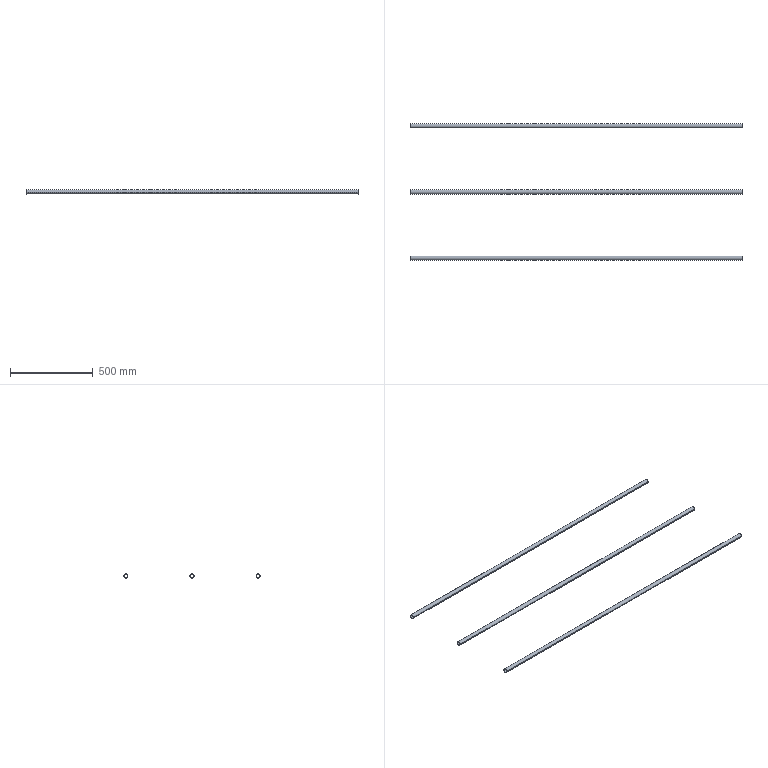Part | STEP file | E3-Transfer kettle guardrail 3 rail_Default<As Machined> | 3 solids | 18 faces | box 2008 x 825 x 25 mm | volume 667105 mm3 | cylinder 12 | plane 6 | commonest cylinder face diameters 22 x6 25 x6
STEP:
#1=CARTESIAN_POINT('',(0.,0.,0.));
#2=DIRECTION('',(0.,0.,1.));
#3=DIRECTION('',(1.,0.,0.));
#4=AXIS2_PLACEMENT_3D('',#1,#2,#3);
#5=CARTESIAN_POINT('',(1004.,787.5,0.));
#6=VERTEX_POINT('',#5);
#7=CARTESIAN_POINT('',(1004.,812.5,0.));
#8=VERTEX_POINT('',#7);
#9=CARTESIAN_POINT('',(1004.,800.,0.));
#10=DIRECTION('',(-1.,0.,0.));
#11=DIRECTION('',(0.,1.,0.));
#12=AXIS2_PLACEMENT_3D('',#9,#10,#11);
#13=CIRCLE('',#12,12.5);
#14=CARTESIAN_POINT('',(1004.,800.,0.));
#15=DIRECTION('',(-1.,0.,0.));
#16=DIRECTION('',(0.,-1.,0.));
#17=AXIS2_PLACEMENT_3D('',#14,#15,#16);
#18=CYLINDRICAL_SURFACE('',#17,12.5);
#19=CARTESIAN_POINT('',(-3.142,0.));
#20=DIRECTION('',(1.,0.));
#21=VECTOR('',#20,1.);
#22=LINE('',#19,#21);
#23=(GEOMETRIC_REPRESENTATION_CONTEXT(2)PARAMETRIC_REPRESENTATION_CONTEXT()REPRESENTATION_CONTEXT('',''));
#24=DEFINITIONAL_REPRESENTATION('',(#22),#23);
#25=PCURVE('',#18,#24);
#26=CARTESIAN_POINT('',(1004.,800.,0.));
#27=DIRECTION('',(1.,0.,0.));
#28=DIRECTION('',(0.,1.,0.));
#29=AXIS2_PLACEMENT_3D('',#26,#27,#28);
#30=PLANE('',#29);
#31=CARTESIAN_POINT('',(12.5,0.));
#32=CARTESIAN_POINT('',(12.5,-21.651));
#33=CARTESIAN_POINT('',(-6.25,-10.825));
#34=CARTESIAN_POINT('',(-25.,0.));
#35=CARTESIAN_POINT('',(-6.25,10.825));
#36=CARTESIAN_POINT('',(12.5,21.651));
#37=CARTESIAN_POINT('',(12.5,0.));
#38=(BOUNDED_CURVE()B_SPLINE_CURVE(2,(#31,#32,#33,#34,#35,#36,#37),.UNSPECIFIED.,.T.,.F.)B_SPLINE_CURVE_WITH_KNOTS((1,2,2,2,2,1),(-2.094,0.,2.094,4.189,6.283,8.378),.UNSPECIFIED.)CURVE()GEOMETRIC_REPRESENTATION_ITEM()RATIONAL_B_SPLINE_CURVE((1.,0.5,1.,0.5,1.,0.5,1.))REPRESENTATION_ITEM(''));
#39=(GEOMETRIC_REPRESENTATION_CONTEXT(2)PARAMETRIC_REPRESENTATION_CONTEXT()REPRESENTATION_CONTEXT('',''));
#40=DEFINITIONAL_REPRESENTATION('',(#38),#39);
#41=PCURVE('',#30,#40);
#42=SURFACE_CURVE('',#13,(#25,#41),.PCURVE_S1.);
#43=EDGE_CURVE('',#6,#8,#42,.T.);
#44=ORIENTED_EDGE('',*,*,#43,.T.);
#45=CARTESIAN_POINT('',(-1004.,812.5,0.));
#46=VERTEX_POINT('',#45);
#47=CARTESIAN_POINT('',(1004.,812.5,0.));
#48=DIRECTION('',(-1.,0.,0.));
#49=VECTOR('',#48,1.);
#50=LINE('',#47,#49);
#51=CARTESIAN_POINT('',(3.142,0.));
#52=DIRECTION('',(0.,1.));
#53=VECTOR('',#52,1.);
#54=LINE('',#51,#53);
#55=(GEOMETRIC_REPRESENTATION_CONTEXT(2)PARAMETRIC_REPRESENTATION_CONTEXT()REPRESENTATION_CONTEXT('',''));
#56=DEFINITIONAL_REPRESENTATION('',(#54),#55);
#57=PCURVE('',#18,#56);
#58=CARTESIAN_POINT('',(1004.,800.,0.));
#59=DIRECTION('',(-1.,0.,0.));
#60=DIRECTION('',(0.,-1.,0.));
#61=AXIS2_PLACEMENT_3D('',#58,#59,#60);
#62=CYLINDRICAL_SURFACE('',#61,12.5);
#63=CARTESIAN_POINT('',(3.142,0.));
#64=DIRECTION('',(0.,1.));
#65=VECTOR('',#64,1.);
#66=LINE('',#63,#65);
#67=(GEOMETRIC_REPRESENTATION_CONTEXT(2)PARAMETRIC_REPRESENTATION_CONTEXT()REPRESENTATION_CONTEXT('',''));
#68=DEFINITIONAL_REPRESENTATION('',(#66),#67);
#69=PCURVE('',#62,#68);
#70=SURFACE_CURVE('',#50,(#57,#69),.PCURVE_S1.);
#71=EDGE_CURVE('',#8,#46,#70,.T.);
#72=ORIENTED_EDGE('',*,*,#71,.T.);
#73=CARTESIAN_POINT('',(-1004.,787.5,0.));
#74=VERTEX_POINT('',#73);
#75=CARTESIAN_POINT('',(-1004.,800.,0.));
#76=DIRECTION('',(-1.,0.,0.));
#77=DIRECTION('',(0.,1.,0.));
#78=AXIS2_PLACEMENT_3D('',#75,#76,#77);
#79=CIRCLE('',#78,12.5);
#80=CARTESIAN_POINT('',(-3.142,2008.));
#81=DIRECTION('',(1.,0.));
#82=VECTOR('',#81,1.);
#83=LINE('',#80,#82);
#84=(GEOMETRIC_REPRESENTATION_CONTEXT(2)PARAMETRIC_REPRESENTATION_CONTEXT()REPRESENTATION_CONTEXT('',''));
#85=DEFINITIONAL_REPRESENTATION('',(#83),#84);
#86=PCURVE('',#18,#85);
#87=CARTESIAN_POINT('',(-1004.,800.,0.));
#88=DIRECTION('',(1.,0.,0.));
#89=DIRECTION('',(0.,1.,0.));
#90=AXIS2_PLACEMENT_3D('',#87,#88,#89);
#91=PLANE('',#90);
#92=CARTESIAN_POINT('',(12.5,0.));
#93=CARTESIAN_POINT('',(12.5,-21.651));
#94=CARTESIAN_POINT('',(-6.25,-10.825));
#95=CARTESIAN_POINT('',(-25.,0.));
#96=CARTESIAN_POINT('',(-6.25,10.825));
#97=CARTESIAN_POINT('',(12.5,21.651));
#98=CARTESIAN_POINT('',(12.5,0.));
#99=(BOUNDED_CURVE()B_SPLINE_CURVE(2,(#92,#93,#94,#95,#96,#97,#98),.UNSPECIFIED.,.T.,.F.)B_SPLINE_CURVE_WITH_KNOTS((1,2,2,2,2,1),(-2.094,0.,2.094,4.189,6.283,8.378),.UNSPECIFIED.)CURVE()GEOMETRIC_REPRESENTATION_ITEM()RATIONAL_B_SPLINE_CURVE((1.,0.5,1.,0.5,1.,0.5,1.))REPRESENTATION_ITEM(''));
#100=(GEOMETRIC_REPRESENTATION_CONTEXT(2)PARAMETRIC_REPRESENTATION_CONTEXT()REPRESENTATION_CONTEXT('',''));
#101=DEFINITIONAL_REPRESENTATION('',(#99),#100);
#102=PCURVE('',#91,#101);
#103=SURFACE_CURVE('',#79,(#86,#102),.PCURVE_S1.);
#104=EDGE_CURVE('',#74,#46,#103,.T.);
#105=ORIENTED_EDGE('',*,*,#104,.F.);
#106=CARTESIAN_POINT('',(1004.,787.5,0.));
#107=DIRECTION('',(-1.,0.,0.));
#108=VECTOR('',#107,1.);
#109=LINE('',#106,#108);
#110=CARTESIAN_POINT('',(0.,0.));
#111=DIRECTION('',(0.,1.));
#112=VECTOR('',#111,1.);
#113=LINE('',#110,#112);
#114=(GEOMETRIC_REPRESENTATION_CONTEXT(2)PARAMETRIC_REPRESENTATION_CONTEXT()REPRESENTATION_CONTEXT('',''));
#115=DEFINITIONAL_REPRESENTATION('',(#113),#114);
#116=PCURVE('',#18,#115);
#117=CARTESIAN_POINT('',(6.283,0.));
#118=DIRECTION('',(0.,1.));
#119=VECTOR('',#118,1.);
#120=LINE('',#117,#119);
#121=(GEOMETRIC_REPRESENTATION_CONTEXT(2)PARAMETRIC_REPRESENTATION_CONTEXT()REPRESENTATION_CONTEXT('',''));
#122=DEFINITIONAL_REPRESENTATION('',(#120),#121);
#123=PCURVE('',#62,#122);
#124=SURFACE_CURVE('',#109,(#116,#123),.PCURVE_S1.);
#125=EDGE_CURVE('',#6,#74,#124,.T.);
#126=ORIENTED_EDGE('',*,*,#125,.F.);
#127=EDGE_LOOP('',(#44,#72,#105,#126));
#128=FACE_BOUND('',#127,.T.);
#129=ADVANCED_FACE('',(#128),#18,.T.);
#130=CARTESIAN_POINT('',(1004.,789.,0.));
#131=VERTEX_POINT('',#130);
#132=CARTESIAN_POINT('',(-1004.,789.,0.));
#133=VERTEX_POINT('',#132);
#134=CARTESIAN_POINT('',(1004.,789.,0.));
#135=DIRECTION('',(-1.,0.,0.));
#136=VECTOR('',#135,1.);
#137=LINE('',#134,#136);
#138=CARTESIAN_POINT('',(1004.,800.,0.));
#139=DIRECTION('',(-1.,0.,0.));
#140=DIRECTION('',(0.,-1.,0.));
#141=AXIS2_PLACEMENT_3D('',#138,#139,#140);
#142=CYLINDRICAL_SURFACE('',#141,11.);
#143=CARTESIAN_POINT('',(6.283,0.));
#144=DIRECTION('',(0.,1.));
#145=VECTOR('',#144,1.);
#146=LINE('',#143,#145);
#147=(GEOMETRIC_REPRESENTATION_CONTEXT(2)PARAMETRIC_REPRESENTATION_CONTEXT()REPRESENTATION_CONTEXT('',''));
#148=DEFINITIONAL_REPRESENTATION('',(#146),#147);
#149=PCURVE('',#142,#148);
#150=CARTESIAN_POINT('',(1004.,800.,0.));
#151=DIRECTION('',(-1.,0.,0.));
#152=DIRECTION('',(0.,-1.,0.));
#153=AXIS2_PLACEMENT_3D('',#150,#151,#152);
#154=CYLINDRICAL_SURFACE('',#153,11.);
#155=CARTESIAN_POINT('',(0.,0.));
#156=DIRECTION('',(0.,1.));
#157=VECTOR('',#156,1.);
#158=LINE('',#155,#157);
#159=(GEOMETRIC_REPRESENTATION_CONTEXT(2)PARAMETRIC_REPRESENTATION_CONTEXT()REPRESENTATION_CONTEXT('',''));
#160=DEFINITIONAL_REPRESENTATION('',(#158),#159);
#161=PCURVE('',#154,#160);
#162=SURFACE_CURVE('',#137,(#149,#161),.PCURVE_S1.);
#163=EDGE_CURVE('',#131,#133,#162,.T.);
#164=ORIENTED_EDGE('',*,*,#163,.T.);
#165=CARTESIAN_POINT('',(-1004.,811.,0.));
#166=VERTEX_POINT('',#165);
#167=CARTESIAN_POINT('',(-1004.,800.,0.));
#168=DIRECTION('',(-1.,0.,0.));
#169=DIRECTION('',(0.,1.,0.));
#170=AXIS2_PLACEMENT_3D('',#167,#168,#169);
#171=CIRCLE('',#170,11.);
#172=CARTESIAN_POINT('',(3.142,2008.));
#173=DIRECTION('',(1.,0.));
#174=VECTOR('',#173,1.);
#175=LINE('',#172,#174);
#176=(GEOMETRIC_REPRESENTATION_CONTEXT(2)PARAMETRIC_REPRESENTATION_CONTEXT()REPRESENTATION_CONTEXT('',''));
#177=DEFINITIONAL_REPRESENTATION('',(#175),#176);
#178=PCURVE('',#142,#177);
#179=CARTESIAN_POINT('',(11.,0.));
#180=CARTESIAN_POINT('',(11.,-19.053));
#181=CARTESIAN_POINT('',(-5.5,-9.526));
#182=CARTESIAN_POINT('',(-22.,0.));
#183=CARTESIAN_POINT('',(-5.5,9.526));
#184=CARTESIAN_POINT('',(11.,19.053));
#185=CARTESIAN_POINT('',(11.,0.));
#186=(BOUNDED_CURVE()B_SPLINE_CURVE(2,(#179,#180,#181,#182,#183,#184,#185),.UNSPECIFIED.,.T.,.F.)B_SPLINE_CURVE_WITH_KNOTS((1,2,2,2,2,1),(-2.094,0.,2.094,4.189,6.283,8.378),.UNSPECIFIED.)CURVE()GEOMETRIC_REPRESENTATION_ITEM()RATIONAL_B_SPLINE_CURVE((1.,0.5,1.,0.5,1.,0.5,1.))REPRESENTATION_ITEM(''));
#187=(GEOMETRIC_REPRESENTATION_CONTEXT(2)PARAMETRIC_REPRESENTATION_CONTEXT()REPRESENTATION_CONTEXT('',''));
#188=DEFINITIONAL_REPRESENTATION('',(#186),#187);
#189=PCURVE('',#91,#188);
#190=SURFACE_CURVE('',#171,(#178,#189),.PCURVE_S1.);
#191=EDGE_CURVE('',#166,#133,#190,.T.);
#192=ORIENTED_EDGE('',*,*,#191,.F.);
#193=CARTESIAN_POINT('',(1004.,811.,0.));
#194=VERTEX_POINT('',#193);
#195=CARTESIAN_POINT('',(1004.,811.,0.));
#196=DIRECTION('',(-1.,0.,0.));
#197=VECTOR('',#196,1.);
#198=LINE('',#195,#197);
#199=CARTESIAN_POINT('',(3.142,0.));
#200=DIRECTION('',(0.,1.));
#201=VECTOR('',#200,1.);
#202=LINE('',#199,#201);
#203=(GEOMETRIC_REPRESENTATION_CONTEXT(2)PARAMETRIC_REPRESENTATION_CONTEXT()REPRESENTATION_CONTEXT('',''));
#204=DEFINITIONAL_REPRESENTATION('',(#202),#203);
#205=PCURVE('',#142,#204);
#206=CARTESIAN_POINT('',(3.142,0.));
#207=DIRECTION('',(0.,1.));
#208=VECTOR('',#207,1.);
#209=LINE('',#206,#208);
#210=(GEOMETRIC_REPRESENTATION_CONTEXT(2)PARAMETRIC_REPRESENTATION_CONTEXT()REPRESENTATION_CONTEXT('',''));
#211=DEFINITIONAL_REPRESENTATION('',(#209),#210);
#212=PCURVE('',#154,#211);
#213=SURFACE_CURVE('',#198,(#205,#212),.PCURVE_S1.);
#214=EDGE_CURVE('',#194,#166,#213,.T.);
#215=ORIENTED_EDGE('',*,*,#214,.F.);
#216=CARTESIAN_POINT('',(1004.,800.,0.));
#217=DIRECTION('',(-1.,0.,0.));
#218=DIRECTION('',(0.,1.,0.));
#219=AXIS2_PLACEMENT_3D('',#216,#217,#218);
#220=CIRCLE('',#219,11.);
#221=CARTESIAN_POINT('',(3.142,0.));
#222=DIRECTION('',(1.,0.));
#223=VECTOR('',#222,1.);
#224=LINE('',#221,#223);
#225=(GEOMETRIC_REPRESENTATION_CONTEXT(2)PARAMETRIC_REPRESENTATION_CONTEXT()REPRESENTATION_CONTEXT('',''));
#226=DEFINITIONAL_REPRESENTATION('',(#224),#225);
#227=PCURVE('',#142,#226);
#228=CARTESIAN_POINT('',(11.,0.));
#229=CARTESIAN_POINT('',(11.,-19.053));
#230=CARTESIAN_POINT('',(-5.5,-9.526));
#231=CARTESIAN_POINT('',(-22.,0.));
#232=CARTESIAN_POINT('',(-5.5,9.526));
#233=CARTESIAN_POINT('',(11.,19.053));
#234=CARTESIAN_POINT('',(11.,0.));
#235=(BOUNDED_CURVE()B_SPLINE_CURVE(2,(#228,#229,#230,#231,#232,#233,#234),.UNSPECIFIED.,.T.,.F.)B_SPLINE_CURVE_WITH_KNOTS((1,2,2,2,2,1),(-2.094,0.,2.094,4.189,6.283,8.378),.UNSPECIFIED.)CURVE()GEOMETRIC_REPRESENTATION_ITEM()RATIONAL_B_SPLINE_CURVE((1.,0.5,1.,0.5,1.,0.5,1.))REPRESENTATION_ITEM(''));
#236=(GEOMETRIC_REPRESENTATION_CONTEXT(2)PARAMETRIC_REPRESENTATION_CONTEXT()REPRESENTATION_CONTEXT('',''));
#237=DEFINITIONAL_REPRESENTATION('',(#235),#236);
#238=PCURVE('',#30,#237);
#239=SURFACE_CURVE('',#220,(#227,#238),.PCURVE_S1.);
#240=EDGE_CURVE('',#194,#131,#239,.T.);
#241=ORIENTED_EDGE('',*,*,#240,.T.);
#242=EDGE_LOOP('',(#164,#192,#215,#241));
#243=FACE_BOUND('',#242,.F.);
#244=ADVANCED_FACE('',(#243),#142,.F.);
#245=CARTESIAN_POINT('',(-1004.,800.,0.));
#246=DIRECTION('',(-1.,0.,0.));
#247=DIRECTION('',(0.,1.,0.));
#248=AXIS2_PLACEMENT_3D('',#245,#246,#247);
#249=CIRCLE('',#248,11.);
#250=CARTESIAN_POINT('',(-3.142,2008.));
#251=DIRECTION('',(1.,0.));
#252=VECTOR('',#251,1.);
#253=LINE('',#250,#252);
#254=(GEOMETRIC_REPRESENTATION_CONTEXT(2)PARAMETRIC_REPRESENTATION_CONTEXT()REPRESENTATION_CONTEXT('',''));
#255=DEFINITIONAL_REPRESENTATION('',(#253),#254);
#256=PCURVE('',#154,#255);
#257=CARTESIAN_POINT('',(11.,0.));
#258=CARTESIAN_POINT('',(11.,-19.053));
#259=CARTESIAN_POINT('',(-5.5,-9.526));
#260=CARTESIAN_POINT('',(-22.,0.));
#261=CARTESIAN_POINT('',(-5.5,9.526));
#262=CARTESIAN_POINT('',(11.,19.053));
#263=CARTESIAN_POINT('',(11.,0.));
#264=(BOUNDED_CURVE()B_SPLINE_CURVE(2,(#257,#258,#259,#260,#261,#262,#263),.UNSPECIFIED.,.T.,.F.)B_SPLINE_CURVE_WITH_KNOTS((1,2,2,2,2,1),(-2.094,0.,2.094,4.189,6.283,8.378),.UNSPECIFIED.)CURVE()GEOMETRIC_REPRESENTATION_ITEM()RATIONAL_B_SPLINE_CURVE((1.,0.5,1.,0.5,1.,0.5,1.))REPRESENTATION_ITEM(''));
#265=(GEOMETRIC_REPRESENTATION_CONTEXT(2)PARAMETRIC_REPRESENTATION_CONTEXT()REPRESENTATION_CONTEXT('',''));
#266=DEFINITIONAL_REPRESENTATION('',(#264),#265);
#267=PCURVE('',#91,#266);
#268=SURFACE_CURVE('',#249,(#256,#267),.PCURVE_S1.);
#269=EDGE_CURVE('',#133,#166,#268,.T.);
#270=ORIENTED_EDGE('',*,*,#269,.F.);
#271=ORIENTED_EDGE('',*,*,#163,.F.);
#272=CARTESIAN_POINT('',(1004.,800.,0.));
#273=DIRECTION('',(-1.,0.,0.));
#274=DIRECTION('',(0.,1.,0.));
#275=AXIS2_PLACEMENT_3D('',#272,#273,#274);
#276=CIRCLE('',#275,11.);
#277=CARTESIAN_POINT('',(-3.142,0.));
#278=DIRECTION('',(1.,0.));
#279=VECTOR('',#278,1.);
#280=LINE('',#277,#279);
#281=(GEOMETRIC_REPRESENTATION_CONTEXT(2)PARAMETRIC_REPRESENTATION_CONTEXT()REPRESENTATION_CONTEXT('',''));
#282=DEFINITIONAL_REPRESENTATION('',(#280),#281);
#283=PCURVE('',#154,#282);
#284=CARTESIAN_POINT('',(11.,0.));
#285=CARTESIAN_POINT('',(11.,-19.053));
#286=CARTESIAN_POINT('',(-5.5,-9.526));
#287=CARTESIAN_POINT('',(-22.,0.));
#288=CARTESIAN_POINT('',(-5.5,9.526));
#289=CARTESIAN_POINT('',(11.,19.053));
#290=CARTESIAN_POINT('',(11.,0.));
#291=(BOUNDED_CURVE()B_SPLINE_CURVE(2,(#284,#285,#286,#287,#288,#289,#290),.UNSPECIFIED.,.T.,.F.)B_SPLINE_CURVE_WITH_KNOTS((1,2,2,2,2,1),(-2.094,0.,2.094,4.189,6.283,8.378),.UNSPECIFIED.)CURVE()GEOMETRIC_REPRESENTATION_ITEM()RATIONAL_B_SPLINE_CURVE((1.,0.5,1.,0.5,1.,0.5,1.))REPRESENTATION_ITEM(''));
#292=(GEOMETRIC_REPRESENTATION_CONTEXT(2)PARAMETRIC_REPRESENTATION_CONTEXT()REPRESENTATION_CONTEXT('',''));
#293=DEFINITIONAL_REPRESENTATION('',(#291),#292);
#294=PCURVE('',#30,#293);
#295=SURFACE_CURVE('',#276,(#283,#294),.PCURVE_S1.);
#296=EDGE_CURVE('',#131,#194,#295,.T.);
#297=ORIENTED_EDGE('',*,*,#296,.T.);
#298=ORIENTED_EDGE('',*,*,#214,.T.);
#299=EDGE_LOOP('',(#270,#271,#297,#298));
#300=FACE_BOUND('',#299,.F.);
#301=ADVANCED_FACE('',(#300),#154,.F.);
#302=ORIENTED_EDGE('',*,*,#71,.F.);
#303=CARTESIAN_POINT('',(1004.,800.,0.));
#304=DIRECTION('',(-1.,0.,0.));
#305=DIRECTION('',(0.,1.,0.));
#306=AXIS2_PLACEMENT_3D('',#303,#304,#305);
#307=CIRCLE('',#306,12.5);
#308=CARTESIAN_POINT('',(3.142,0.));
#309=DIRECTION('',(1.,0.));
#310=VECTOR('',#309,1.);
#311=LINE('',#308,#310);
#312=(GEOMETRIC_REPRESENTATION_CONTEXT(2)PARAMETRIC_REPRESENTATION_CONTEXT()REPRESENTATION_CONTEXT('',''));
#313=DEFINITIONAL_REPRESENTATION('',(#311),#312);
#314=PCURVE('',#62,#313);
#315=CARTESIAN_POINT('',(12.5,0.));
#316=CARTESIAN_POINT('',(12.5,-21.651));
#317=CARTESIAN_POINT('',(-6.25,-10.825));
#318=CARTESIAN_POINT('',(-25.,0.));
#319=CARTESIAN_POINT('',(-6.25,10.825));
#320=CARTESIAN_POINT('',(12.5,21.651));
#321=CARTESIAN_POINT('',(12.5,0.));
#322=(BOUNDED_CURVE()B_SPLINE_CURVE(2,(#315,#316,#317,#318,#319,#320,#321),.UNSPECIFIED.,.T.,.F.)B_SPLINE_CURVE_WITH_KNOTS((1,2,2,2,2,1),(-2.094,0.,2.094,4.189,6.283,8.378),.UNSPECIFIED.)CURVE()GEOMETRIC_REPRESENTATION_ITEM()RATIONAL_B_SPLINE_CURVE((1.,0.5,1.,0.5,1.,0.5,1.))REPRESENTATION_ITEM(''));
#323=(GEOMETRIC_REPRESENTATION_CONTEXT(2)PARAMETRIC_REPRESENTATION_CONTEXT()REPRESENTATION_CONTEXT('',''));
#324=DEFINITIONAL_REPRESENTATION('',(#322),#323);
#325=PCURVE('',#30,#324);
#326=SURFACE_CURVE('',#307,(#314,#325),.PCURVE_S1.);
#327=EDGE_CURVE('',#8,#6,#326,.T.);
#328=ORIENTED_EDGE('',*,*,#327,.T.);
#329=ORIENTED_EDGE('',*,*,#125,.T.);
#330=CARTESIAN_POINT('',(-1004.,800.,0.));
#331=DIRECTION('',(-1.,0.,0.));
#332=DIRECTION('',(0.,1.,0.));
#333=AXIS2_PLACEMENT_3D('',#330,#331,#332);
#334=CIRCLE('',#333,12.5);
#335=CARTESIAN_POINT('',(3.142,2008.));
#336=DIRECTION('',(1.,0.));
#337=VECTOR('',#336,1.);
#338=LINE('',#335,#337);
#339=(GEOMETRIC_REPRESENTATION_CONTEXT(2)PARAMETRIC_REPRESENTATION_CONTEXT()REPRESENTATION_CONTEXT('',''));
#340=DEFINITIONAL_REPRESENTATION('',(#338),#339);
#341=PCURVE('',#62,#340);
#342=CARTESIAN_POINT('',(12.5,0.));
#343=CARTESIAN_POINT('',(12.5,-21.651));
#344=CARTESIAN_POINT('',(-6.25,-10.825));
#345=CARTESIAN_POINT('',(-25.,0.));
#346=CARTESIAN_POINT('',(-6.25,10.825));
#347=CARTESIAN_POINT('',(12.5,21.651));
#348=CARTESIAN_POINT('',(12.5,0.));
#349=(BOUNDED_CURVE()B_SPLINE_CURVE(2,(#342,#343,#344,#345,#346,#347,#348),.UNSPECIFIED.,.T.,.F.)B_SPLINE_CURVE_WITH_KNOTS((1,2,2,2,2,1),(-2.094,0.,2.094,4.189,6.283,8.378),.UNSPECIFIED.)CURVE()GEOMETRIC_REPRESENTATION_ITEM()RATIONAL_B_SPLINE_CURVE((1.,0.5,1.,0.5,1.,0.5,1.))REPRESENTATION_ITEM(''));
#350=(GEOMETRIC_REPRESENTATION_CONTEXT(2)PARAMETRIC_REPRESENTATION_CONTEXT()REPRESENTATION_CONTEXT('',''));
#351=DEFINITIONAL_REPRESENTATION('',(#349),#350);
#352=PCURVE('',#91,#351);
#353=SURFACE_CURVE('',#334,(#341,#352),.PCURVE_S1.);
#354=EDGE_CURVE('',#46,#74,#353,.T.);
#355=ORIENTED_EDGE('',*,*,#354,.F.);
#356=EDGE_LOOP('',(#302,#328,#329,#355));
#357=FACE_BOUND('',#356,.T.);
#358=ADVANCED_FACE('',(#357),#62,.T.);
#359=ORIENTED_EDGE('',*,*,#296,.T.);
#360=ORIENTED_EDGE('',*,*,#240,.T.);
#361=EDGE_LOOP('',(#359,#360));
#362=FACE_BOUND('',#361,.T.);
#363=ORIENTED_EDGE('',*,*,#43,.F.);
#364=ORIENTED_EDGE('',*,*,#327,.F.);
#365=EDGE_LOOP('',(#363,#364));
#366=FACE_BOUND('',#365,.T.);
#367=ADVANCED_FACE('',(#362,#366),#30,.T.);
#368=ORIENTED_EDGE('',*,*,#269,.F.);
#369=ORIENTED_EDGE('',*,*,#191,.F.);
#370=EDGE_LOOP('',(#368,#369));
#371=FACE_BOUND('',#370,.T.);
#372=ORIENTED_EDGE('',*,*,#104,.T.);
#373=ORIENTED_EDGE('',*,*,#354,.T.);
#374=EDGE_LOOP('',(#372,#373));
#375=FACE_BOUND('',#374,.T.);
#376=ADVANCED_FACE('',(#371,#375),#91,.F.);
#377=CLOSED_SHELL('',(#129,#244,#301,#358,#367,#376));
#378=MANIFOLD_SOLID_BREP('',#377);
#379=CARTESIAN_POINT('',(1004.,-12.5,0.));
#380=VERTEX_POINT('',#379);
#381=CARTESIAN_POINT('',(1004.,12.5,0.));
#382=VERTEX_POINT('',#381);
#383=CARTESIAN_POINT('',(1004.,0.,0.));
#384=DIRECTION('',(-1.,0.,0.));
#385=DIRECTION('',(0.,1.,0.));
#386=AXIS2_PLACEMENT_3D('',#383,#384,#385);
#387=CIRCLE('',#386,12.5);
#388=CARTESIAN_POINT('',(1004.,0.,0.));
#389=DIRECTION('',(-1.,0.,0.));
#390=DIRECTION('',(0.,-1.,0.));
#391=AXIS2_PLACEMENT_3D('',#388,#389,#390);
#392=CYLINDRICAL_SURFACE('',#391,12.5);
#393=CARTESIAN_POINT('',(-3.142,0.));
#394=DIRECTION('',(1.,0.));
#395=VECTOR('',#394,1.);
#396=LINE('',#393,#395);
#397=(GEOMETRIC_REPRESENTATION_CONTEXT(2)PARAMETRIC_REPRESENTATION_CONTEXT()REPRESENTATION_CONTEXT('',''));
#398=DEFINITIONAL_REPRESENTATION('',(#396),#397);
#399=PCURVE('',#392,#398);
#400=CARTESIAN_POINT('',(1004.,0.,0.));
#401=DIRECTION('',(1.,0.,0.));
#402=DIRECTION('',(0.,1.,0.));
#403=AXIS2_PLACEMENT_3D('',#400,#401,#402);
#404=PLANE('',#403);
#405=CARTESIAN_POINT('',(12.5,0.));
#406=CARTESIAN_POINT('',(12.5,-21.651));
#407=CARTESIAN_POINT('',(-6.25,-10.825));
#408=CARTESIAN_POINT('',(-25.,0.));
#409=CARTESIAN_POINT('',(-6.25,10.825));
#410=CARTESIAN_POINT('',(12.5,21.651));
#411=CARTESIAN_POINT('',(12.5,0.));
#412=(BOUNDED_CURVE()B_SPLINE_CURVE(2,(#405,#406,#407,#408,#409,#410,#411),.UNSPECIFIED.,.T.,.F.)B_SPLINE_CURVE_WITH_KNOTS((1,2,2,2,2,1),(-2.094,0.,2.094,4.189,6.283,8.378),.UNSPECIFIED.)CURVE()GEOMETRIC_REPRESENTATION_ITEM()RATIONAL_B_SPLINE_CURVE((1.,0.5,1.,0.5,1.,0.5,1.))REPRESENTATION_ITEM(''));
#413=(GEOMETRIC_REPRESENTATION_CONTEXT(2)PARAMETRIC_REPRESENTATION_CONTEXT()REPRESENTATION_CONTEXT('',''));
#414=DEFINITIONAL_REPRESENTATION('',(#412),#413);
#415=PCURVE('',#404,#414);
#416=SURFACE_CURVE('',#387,(#399,#415),.PCURVE_S1.);
#417=EDGE_CURVE('',#380,#382,#416,.T.);
#418=ORIENTED_EDGE('',*,*,#417,.T.);
#419=CARTESIAN_POINT('',(-1004.,12.5,0.));
#420=VERTEX_POINT('',#419);
#421=CARTESIAN_POINT('',(1004.,12.5,0.));
#422=DIRECTION('',(-1.,0.,0.));
#423=VECTOR('',#422,1.);
#424=LINE('',#421,#423);
#425=CARTESIAN_POINT('',(3.142,0.));
#426=DIRECTION('',(0.,1.));
#427=VECTOR('',#426,1.);
#428=LINE('',#425,#427);
#429=(GEOMETRIC_REPRESENTATION_CONTEXT(2)PARAMETRIC_REPRESENTATION_CONTEXT()REPRESENTATION_CONTEXT('',''));
#430=DEFINITIONAL_REPRESENTATION('',(#428),#429);
#431=PCURVE('',#392,#430);
#432=CARTESIAN_POINT('',(1004.,0.,0.));
#433=DIRECTION('',(-1.,0.,0.));
#434=DIRECTION('',(0.,-1.,0.));
#435=AXIS2_PLACEMENT_3D('',#432,#433,#434);
#436=CYLINDRICAL_SURFACE('',#435,12.5);
#437=CARTESIAN_POINT('',(3.142,0.));
#438=DIRECTION('',(0.,1.));
#439=VECTOR('',#438,1.);
#440=LINE('',#437,#439);
#441=(GEOMETRIC_REPRESENTATION_CONTEXT(2)PARAMETRIC_REPRESENTATION_CONTEXT()REPRESENTATION_CONTEXT('',''));
#442=DEFINITIONAL_REPRESENTATION('',(#440),#441);
#443=PCURVE('',#436,#442);
#444=SURFACE_CURVE('',#424,(#431,#443),.PCURVE_S1.);
#445=EDGE_CURVE('',#382,#420,#444,.T.);
#446=ORIENTED_EDGE('',*,*,#445,.T.);
#447=CARTESIAN_POINT('',(-1004.,-12.5,0.));
#448=VERTEX_POINT('',#447);
#449=CARTESIAN_POINT('',(-1004.,0.,0.));
#450=DIRECTION('',(-1.,0.,0.));
#451=DIRECTION('',(0.,1.,0.));
#452=AXIS2_PLACEMENT_3D('',#449,#450,#451);
#453=CIRCLE('',#452,12.5);
#454=CARTESIAN_POINT('',(-3.142,2008.));
#455=DIRECTION('',(1.,0.));
#456=VECTOR('',#455,1.);
#457=LINE('',#454,#456);
#458=(GEOMETRIC_REPRESENTATION_CONTEXT(2)PARAMETRIC_REPRESENTATION_CONTEXT()REPRESENTATION_CONTEXT('',''));
#459=DEFINITIONAL_REPRESENTATION('',(#457),#458);
#460=PCURVE('',#392,#459);
#461=CARTESIAN_POINT('',(-1004.,0.,0.));
#462=DIRECTION('',(1.,0.,0.));
#463=DIRECTION('',(0.,1.,0.));
#464=AXIS2_PLACEMENT_3D('',#461,#462,#463);
#465=PLANE('',#464);
#466=CARTESIAN_POINT('',(12.5,0.));
#467=CARTESIAN_POINT('',(12.5,-21.651));
#468=CARTESIAN_POINT('',(-6.25,-10.825));
#469=CARTESIAN_POINT('',(-25.,0.));
#470=CARTESIAN_POINT('',(-6.25,10.825));
#471=CARTESIAN_POINT('',(12.5,21.651));
#472=CARTESIAN_POINT('',(12.5,0.));
#473=(BOUNDED_CURVE()B_SPLINE_CURVE(2,(#466,#467,#468,#469,#470,#471,#472),.UNSPECIFIED.,.T.,.F.)B_SPLINE_CURVE_WITH_KNOTS((1,2,2,2,2,1),(-2.094,0.,2.094,4.189,6.283,8.378),.UNSPECIFIED.)CURVE()GEOMETRIC_REPRESENTATION_ITEM()RATIONAL_B_SPLINE_CURVE((1.,0.5,1.,0.5,1.,0.5,1.))REPRESENTATION_ITEM(''));
#474=(GEOMETRIC_REPRESENTATION_CONTEXT(2)PARAMETRIC_REPRESENTATION_CONTEXT()REPRESENTATION_CONTEXT('',''));
#475=DEFINITIONAL_REPRESENTATION('',(#473),#474);
#476=PCURVE('',#465,#475);
#477=SURFACE_CURVE('',#453,(#460,#476),.PCURVE_S1.);
#478=EDGE_CURVE('',#448,#420,#477,.T.);
#479=ORIENTED_EDGE('',*,*,#478,.F.);
#480=CARTESIAN_POINT('',(1004.,-12.5,0.));
#481=DIRECTION('',(-1.,0.,0.));
#482=VECTOR('',#481,1.);
#483=LINE('',#480,#482);
#484=CARTESIAN_POINT('',(0.,0.));
#485=DIRECTION('',(0.,1.));
#486=VECTOR('',#485,1.);
#487=LINE('',#484,#486);
#488=(GEOMETRIC_REPRESENTATION_CONTEXT(2)PARAMETRIC_REPRESENTATION_CONTEXT()REPRESENTATION_CONTEXT('',''));
#489=DEFINITIONAL_REPRESENTATION('',(#487),#488);
#490=PCURVE('',#392,#489);
#491=CARTESIAN_POINT('',(6.283,0.));
#492=DIRECTION('',(0.,1.));
#493=VECTOR('',#492,1.);
#494=LINE('',#491,#493);
#495=(GEOMETRIC_REPRESENTATION_CONTEXT(2)PARAMETRIC_REPRESENTATION_CONTEXT()REPRESENTATION_CONTEXT('',''));
#496=DEFINITIONAL_REPRESENTATION('',(#494),#495);
#497=PCURVE('',#436,#496);
#498=SURFACE_CURVE('',#483,(#490,#497),.PCURVE_S1.);
#499=EDGE_CURVE('',#380,#448,#498,.T.);
#500=ORIENTED_EDGE('',*,*,#499,.F.);
#501=EDGE_LOOP('',(#418,#446,#479,#500));
#502=FACE_BOUND('',#501,.T.);
#503=ADVANCED_FACE('',(#502),#392,.T.);
#504=CARTESIAN_POINT('',(1004.,-11.,0.));
#505=VERTEX_POINT('',#504);
#506=CARTESIAN_POINT('',(-1004.,-11.,0.));
#507=VERTEX_POINT('',#506);
#508=CARTESIAN_POINT('',(1004.,-11.,0.));
#509=DIRECTION('',(-1.,0.,0.));
#510=VECTOR('',#509,1.);
#511=LINE('',#508,#510);
#512=CARTESIAN_POINT('',(1004.,0.,0.));
#513=DIRECTION('',(-1.,0.,0.));
#514=DIRECTION('',(0.,-1.,0.));
#515=AXIS2_PLACEMENT_3D('',#512,#513,#514);
#516=CYLINDRICAL_SURFACE('',#515,11.);
#517=CARTESIAN_POINT('',(6.283,0.));
#518=DIRECTION('',(0.,1.));
#519=VECTOR('',#518,1.);
#520=LINE('',#517,#519);
#521=(GEOMETRIC_REPRESENTATION_CONTEXT(2)PARAMETRIC_REPRESENTATION_CONTEXT()REPRESENTATION_CONTEXT('',''));
#522=DEFINITIONAL_REPRESENTATION('',(#520),#521);
#523=PCURVE('',#516,#522);
#524=CARTESIAN_POINT('',(1004.,0.,0.));
#525=DIRECTION('',(-1.,0.,0.));
#526=DIRECTION('',(0.,-1.,0.));
#527=AXIS2_PLACEMENT_3D('',#524,#525,#526);
#528=CYLINDRICAL_SURFACE('',#527,11.);
#529=CARTESIAN_POINT('',(0.,0.));
#530=DIRECTION('',(0.,1.));
#531=VECTOR('',#530,1.);
#532=LINE('',#529,#531);
#533=(GEOMETRIC_REPRESENTATION_CONTEXT(2)PARAMETRIC_REPRESENTATION_CONTEXT()REPRESENTATION_CONTEXT('',''));
#534=DEFINITIONAL_REPRESENTATION('',(#532),#533);
#535=PCURVE('',#528,#534);
#536=SURFACE_CURVE('',#511,(#523,#535),.PCURVE_S1.);
#537=EDGE_CURVE('',#505,#507,#536,.T.);
#538=ORIENTED_EDGE('',*,*,#537,.T.);
#539=CARTESIAN_POINT('',(-1004.,11.,0.));
#540=VERTEX_POINT('',#539);
#541=CARTESIAN_POINT('',(-1004.,0.,0.));
#542=DIRECTION('',(-1.,0.,0.));
#543=DIRECTION('',(0.,1.,0.));
#544=AXIS2_PLACEMENT_3D('',#541,#542,#543);
#545=CIRCLE('',#544,11.);
#546=CARTESIAN_POINT('',(3.142,2008.));
#547=DIRECTION('',(1.,0.));
#548=VECTOR('',#547,1.);
#549=LINE('',#546,#548);
#550=(GEOMETRIC_REPRESENTATION_CONTEXT(2)PARAMETRIC_REPRESENTATION_CONTEXT()REPRESENTATION_CONTEXT('',''));
#551=DEFINITIONAL_REPRESENTATION('',(#549),#550);
#552=PCURVE('',#516,#551);
#553=CARTESIAN_POINT('',(11.,0.));
#554=CARTESIAN_POINT('',(11.,-19.053));
#555=CARTESIAN_POINT('',(-5.5,-9.526));
#556=CARTESIAN_POINT('',(-22.,0.));
#557=CARTESIAN_POINT('',(-5.5,9.526));
#558=CARTESIAN_POINT('',(11.,19.053));
#559=CARTESIAN_POINT('',(11.,0.));
#560=(BOUNDED_CURVE()B_SPLINE_CURVE(2,(#553,#554,#555,#556,#557,#558,#559),.UNSPECIFIED.,.T.,.F.)B_SPLINE_CURVE_WITH_KNOTS((1,2,2,2,2,1),(-2.094,0.,2.094,4.189,6.283,8.378),.UNSPECIFIED.)CURVE()GEOMETRIC_REPRESENTATION_ITEM()RATIONAL_B_SPLINE_CURVE((1.,0.5,1.,0.5,1.,0.5,1.))REPRESENTATION_ITEM(''));
#561=(GEOMETRIC_REPRESENTATION_CONTEXT(2)PARAMETRIC_REPRESENTATION_CONTEXT()REPRESENTATION_CONTEXT('',''));
#562=DEFINITIONAL_REPRESENTATION('',(#560),#561);
#563=PCURVE('',#465,#562);
#564=SURFACE_CURVE('',#545,(#552,#563),.PCURVE_S1.);
#565=EDGE_CURVE('',#540,#507,#564,.T.);
#566=ORIENTED_EDGE('',*,*,#565,.F.);
#567=CARTESIAN_POINT('',(1004.,11.,0.));
#568=VERTEX_POINT('',#567);
#569=CARTESIAN_POINT('',(1004.,11.,0.));
#570=DIRECTION('',(-1.,0.,0.));
#571=VECTOR('',#570,1.);
#572=LINE('',#569,#571);
#573=CARTESIAN_POINT('',(3.142,0.));
#574=DIRECTION('',(0.,1.));
#575=VECTOR('',#574,1.);
#576=LINE('',#573,#575);
#577=(GEOMETRIC_REPRESENTATION_CONTEXT(2)PARAMETRIC_REPRESENTATION_CONTEXT()REPRESENTATION_CONTEXT('',''));
#578=DEFINITIONAL_REPRESENTATION('',(#576),#577);
#579=PCURVE('',#516,#578);
#580=CARTESIAN_POINT('',(3.142,0.));
#581=DIRECTION('',(0.,1.));
#582=VECTOR('',#581,1.);
#583=LINE('',#580,#582);
#584=(GEOMETRIC_REPRESENTATION_CONTEXT(2)PARAMETRIC_REPRESENTATION_CONTEXT()REPRESENTATION_CONTEXT('',''));
#585=DEFINITIONAL_REPRESENTATION('',(#583),#584);
#586=PCURVE('',#528,#585);
#587=SURFACE_CURVE('',#572,(#579,#586),.PCURVE_S1.);
#588=EDGE_CURVE('',#568,#540,#587,.T.);
#589=ORIENTED_EDGE('',*,*,#588,.F.);
#590=CARTESIAN_POINT('',(1004.,0.,0.));
#591=DIRECTION('',(-1.,0.,0.));
#592=DIRECTION('',(0.,1.,0.));
#593=AXIS2_PLACEMENT_3D('',#590,#591,#592);
#594=CIRCLE('',#593,11.);
#595=CARTESIAN_POINT('',(3.142,0.));
#596=DIRECTION('',(1.,0.));
#597=VECTOR('',#596,1.);
#598=LINE('',#595,#597);
#599=(GEOMETRIC_REPRESENTATION_CONTEXT(2)PARAMETRIC_REPRESENTATION_CONTEXT()REPRESENTATION_CONTEXT('',''));
#600=DEFINITIONAL_REPRESENTATION('',(#598),#599);
#601=PCURVE('',#516,#600);
#602=CARTESIAN_POINT('',(11.,0.));
#603=CARTESIAN_POINT('',(11.,-19.053));
#604=CARTESIAN_POINT('',(-5.5,-9.526));
#605=CARTESIAN_POINT('',(-22.,0.));
#606=CARTESIAN_POINT('',(-5.5,9.526));
#607=CARTESIAN_POINT('',(11.,19.053));
#608=CARTESIAN_POINT('',(11.,0.));
#609=(BOUNDED_CURVE()B_SPLINE_CURVE(2,(#602,#603,#604,#605,#606,#607,#608),.UNSPECIFIED.,.T.,.F.)B_SPLINE_CURVE_WITH_KNOTS((1,2,2,2,2,1),(-2.094,0.,2.094,4.189,6.283,8.378),.UNSPECIFIED.)CURVE()GEOMETRIC_REPRESENTATION_ITEM()RATIONAL_B_SPLINE_CURVE((1.,0.5,1.,0.5,1.,0.5,1.))REPRESENTATION_ITEM(''));
#610=(GEOMETRIC_REPRESENTATION_CONTEXT(2)PARAMETRIC_REPRESENTATION_CONTEXT()REPRESENTATION_CONTEXT('',''));
#611=DEFINITIONAL_REPRESENTATION('',(#609),#610);
#612=PCURVE('',#404,#611);
#613=SURFACE_CURVE('',#594,(#601,#612),.PCURVE_S1.);
#614=EDGE_CURVE('',#568,#505,#613,.T.);
#615=ORIENTED_EDGE('',*,*,#614,.T.);
#616=EDGE_LOOP('',(#538,#566,#589,#615));
#617=FACE_BOUND('',#616,.F.);
#618=ADVANCED_FACE('',(#617),#516,.F.);
#619=CARTESIAN_POINT('',(-1004.,0.,0.));
#620=DIRECTION('',(-1.,0.,0.));
#621=DIRECTION('',(0.,1.,0.));
#622=AXIS2_PLACEMENT_3D('',#619,#620,#621);
#623=CIRCLE('',#622,11.);
#624=CARTESIAN_POINT('',(-3.142,2008.));
#625=DIRECTION('',(1.,0.));
#626=VECTOR('',#625,1.);
#627=LINE('',#624,#626);
#628=(GEOMETRIC_REPRESENTATION_CONTEXT(2)PARAMETRIC_REPRESENTATION_CONTEXT()REPRESENTATION_CONTEXT('',''));
#629=DEFINITIONAL_REPRESENTATION('',(#627),#628);
#630=PCURVE('',#528,#629);
#631=CARTESIAN_POINT('',(11.,0.));
#632=CARTESIAN_POINT('',(11.,-19.053));
#633=CARTESIAN_POINT('',(-5.5,-9.526));
#634=CARTESIAN_POINT('',(-22.,0.));
#635=CARTESIAN_POINT('',(-5.5,9.526));
#636=CARTESIAN_POINT('',(11.,19.053));
#637=CARTESIAN_POINT('',(11.,0.));
#638=(BOUNDED_CURVE()B_SPLINE_CURVE(2,(#631,#632,#633,#634,#635,#636,#637),.UNSPECIFIED.,.T.,.F.)B_SPLINE_CURVE_WITH_KNOTS((1,2,2,2,2,1),(-2.094,0.,2.094,4.189,6.283,8.378),.UNSPECIFIED.)CURVE()GEOMETRIC_REPRESENTATION_ITEM()RATIONAL_B_SPLINE_CURVE((1.,0.5,1.,0.5,1.,0.5,1.))REPRESENTATION_ITEM(''));
#639=(GEOMETRIC_REPRESENTATION_CONTEXT(2)PARAMETRIC_REPRESENTATION_CONTEXT()REPRESENTATION_CONTEXT('',''));
#640=DEFINITIONAL_REPRESENTATION('',(#638),#639);
#641=PCURVE('',#465,#640);
#642=SURFACE_CURVE('',#623,(#630,#641),.PCURVE_S1.);
#643=EDGE_CURVE('',#507,#540,#642,.T.);
#644=ORIENTED_EDGE('',*,*,#643,.F.);
#645=ORIENTED_EDGE('',*,*,#537,.F.);
#646=CARTESIAN_POINT('',(1004.,0.,0.));
#647=DIRECTION('',(-1.,0.,0.));
#648=DIRECTION('',(0.,1.,0.));
#649=AXIS2_PLACEMENT_3D('',#646,#647,#648);
#650=CIRCLE('',#649,11.);
#651=CARTESIAN_POINT('',(-3.142,0.));
#652=DIRECTION('',(1.,0.));
#653=VECTOR('',#652,1.);
#654=LINE('',#651,#653);
#655=(GEOMETRIC_REPRESENTATION_CONTEXT(2)PARAMETRIC_REPRESENTATION_CONTEXT()REPRESENTATION_CONTEXT('',''));
#656=DEFINITIONAL_REPRESENTATION('',(#654),#655);
#657=PCURVE('',#528,#656);
#658=CARTESIAN_POINT('',(11.,0.));
#659=CARTESIAN_POINT('',(11.,-19.053));
#660=CARTESIAN_POINT('',(-5.5,-9.526));
#661=CARTESIAN_POINT('',(-22.,0.));
#662=CARTESIAN_POINT('',(-5.5,9.526));
#663=CARTESIAN_POINT('',(11.,19.053));
#664=CARTESIAN_POINT('',(11.,0.));
#665=(BOUNDED_CURVE()B_SPLINE_CURVE(2,(#658,#659,#660,#661,#662,#663,#664),.UNSPECIFIED.,.T.,.F.)B_SPLINE_CURVE_WITH_KNOTS((1,2,2,2,2,1),(-2.094,0.,2.094,4.189,6.283,8.378),.UNSPECIFIED.)CURVE()GEOMETRIC_REPRESENTATION_ITEM()RATIONAL_B_SPLINE_CURVE((1.,0.5,1.,0.5,1.,0.5,1.))REPRESENTATION_ITEM(''));
#666=(GEOMETRIC_REPRESENTATION_CONTEXT(2)PARAMETRIC_REPRESENTATION_CONTEXT()REPRESENTATION_CONTEXT('',''));
#667=DEFINITIONAL_REPRESENTATION('',(#665),#666);
#668=PCURVE('',#404,#667);
#669=SURFACE_CURVE('',#650,(#657,#668),.PCURVE_S1.);
#670=EDGE_CURVE('',#505,#568,#669,.T.);
#671=ORIENTED_EDGE('',*,*,#670,.T.);
#672=ORIENTED_EDGE('',*,*,#588,.T.);
#673=EDGE_LOOP('',(#644,#645,#671,#672));
#674=FACE_BOUND('',#673,.F.);
#675=ADVANCED_FACE('',(#674),#528,.F.);
#676=ORIENTED_EDGE('',*,*,#445,.F.);
#677=CARTESIAN_POINT('',(1004.,0.,0.));
#678=DIRECTION('',(-1.,0.,0.));
#679=DIRECTION('',(0.,1.,0.));
#680=AXIS2_PLACEMENT_3D('',#677,#678,#679);
#681=CIRCLE('',#680,12.5);
#682=CARTESIAN_POINT('',(3.142,0.));
#683=DIRECTION('',(1.,0.));
#684=VECTOR('',#683,1.);
#685=LINE('',#682,#684);
#686=(GEOMETRIC_REPRESENTATION_CONTEXT(2)PARAMETRIC_REPRESENTATION_CONTEXT()REPRESENTATION_CONTEXT('',''));
#687=DEFINITIONAL_REPRESENTATION('',(#685),#686);
#688=PCURVE('',#436,#687);
#689=CARTESIAN_POINT('',(12.5,0.));
#690=CARTESIAN_POINT('',(12.5,-21.651));
#691=CARTESIAN_POINT('',(-6.25,-10.825));
#692=CARTESIAN_POINT('',(-25.,0.));
#693=CARTESIAN_POINT('',(-6.25,10.825));
#694=CARTESIAN_POINT('',(12.5,21.651));
#695=CARTESIAN_POINT('',(12.5,0.));
#696=(BOUNDED_CURVE()B_SPLINE_CURVE(2,(#689,#690,#691,#692,#693,#694,#695),.UNSPECIFIED.,.T.,.F.)B_SPLINE_CURVE_WITH_KNOTS((1,2,2,2,2,1),(-2.094,0.,2.094,4.189,6.283,8.378),.UNSPECIFIED.)CURVE()GEOMETRIC_REPRESENTATION_ITEM()RATIONAL_B_SPLINE_CURVE((1.,0.5,1.,0.5,1.,0.5,1.))REPRESENTATION_ITEM(''));
#697=(GEOMETRIC_REPRESENTATION_CONTEXT(2)PARAMETRIC_REPRESENTATION_CONTEXT()REPRESENTATION_CONTEXT('',''));
#698=DEFINITIONAL_REPRESENTATION('',(#696),#697);
#699=PCURVE('',#404,#698);
#700=SURFACE_CURVE('',#681,(#688,#699),.PCURVE_S1.);
#701=EDGE_CURVE('',#382,#380,#700,.T.);
#702=ORIENTED_EDGE('',*,*,#701,.T.);
#703=ORIENTED_EDGE('',*,*,#499,.T.);
#704=CARTESIAN_POINT('',(-1004.,0.,0.));
#705=DIRECTION('',(-1.,0.,0.));
#706=DIRECTION('',(0.,1.,0.));
#707=AXIS2_PLACEMENT_3D('',#704,#705,#706);
#708=CIRCLE('',#707,12.5);
#709=CARTESIAN_POINT('',(3.142,2008.));
#710=DIRECTION('',(1.,0.));
#711=VECTOR('',#710,1.);
#712=LINE('',#709,#711);
#713=(GEOMETRIC_REPRESENTATION_CONTEXT(2)PARAMETRIC_REPRESENTATION_CONTEXT()REPRESENTATION_CONTEXT('',''));
#714=DEFINITIONAL_REPRESENTATION('',(#712),#713);
#715=PCURVE('',#436,#714);
#716=CARTESIAN_POINT('',(12.5,0.));
#717=CARTESIAN_POINT('',(12.5,-21.651));
#718=CARTESIAN_POINT('',(-6.25,-10.825));
#719=CARTESIAN_POINT('',(-25.,0.));
#720=CARTESIAN_POINT('',(-6.25,10.825));
#721=CARTESIAN_POINT('',(12.5,21.651));
#722=CARTESIAN_POINT('',(12.5,0.));
#723=(BOUNDED_CURVE()B_SPLINE_CURVE(2,(#716,#717,#718,#719,#720,#721,#722),.UNSPECIFIED.,.T.,.F.)B_SPLINE_CURVE_WITH_KNOTS((1,2,2,2,2,1),(-2.094,0.,2.094,4.189,6.283,8.378),.UNSPECIFIED.)CURVE()GEOMETRIC_REPRESENTATION_ITEM()RATIONAL_B_SPLINE_CURVE((1.,0.5,1.,0.5,1.,0.5,1.))REPRESENTATION_ITEM(''));
#724=(GEOMETRIC_REPRESENTATION_CONTEXT(2)PARAMETRIC_REPRESENTATION_CONTEXT()REPRESENTATION_CONTEXT('',''));
#725=DEFINITIONAL_REPRESENTATION('',(#723),#724);
#726=PCURVE('',#465,#725);
#727=SURFACE_CURVE('',#708,(#715,#726),.PCURVE_S1.);
#728=EDGE_CURVE('',#420,#448,#727,.T.);
#729=ORIENTED_EDGE('',*,*,#728,.F.);
#730=EDGE_LOOP('',(#676,#702,#703,#729));
#731=FACE_BOUND('',#730,.T.);
#732=ADVANCED_FACE('',(#731),#436,.T.);
#733=ORIENTED_EDGE('',*,*,#670,.T.);
#734=ORIENTED_EDGE('',*,*,#614,.T.);
#735=EDGE_LOOP('',(#733,#734));
#736=FACE_BOUND('',#735,.T.);
#737=ORIENTED_EDGE('',*,*,#417,.F.);
#738=ORIENTED_EDGE('',*,*,#701,.F.);
#739=EDGE_LOOP('',(#737,#738));
#740=FACE_BOUND('',#739,.T.);
#741=ADVANCED_FACE('',(#736,#740),#404,.T.);
#742=ORIENTED_EDGE('',*,*,#643,.F.);
#743=ORIENTED_EDGE('',*,*,#565,.F.);
#744=EDGE_LOOP('',(#742,#743));
#745=FACE_BOUND('',#744,.T.);
#746=ORIENTED_EDGE('',*,*,#478,.T.);
#747=ORIENTED_EDGE('',*,*,#728,.T.);
#748=EDGE_LOOP('',(#746,#747));
#749=FACE_BOUND('',#748,.T.);
#750=ADVANCED_FACE('',(#745,#749),#465,.F.);
#751=CLOSED_SHELL('',(#503,#618,#675,#732,#741,#750));
#752=MANIFOLD_SOLID_BREP('',#751);
#753=CARTESIAN_POINT('',(1004.,387.5,0.));
#754=VERTEX_POINT('',#753);
#755=CARTESIAN_POINT('',(1004.,412.5,0.));
#756=VERTEX_POINT('',#755);
#757=CARTESIAN_POINT('',(1004.,400.,0.));
#758=DIRECTION('',(-1.,0.,0.));
#759=DIRECTION('',(0.,1.,0.));
#760=AXIS2_PLACEMENT_3D('',#757,#758,#759);
#761=CIRCLE('',#760,12.5);
#762=CARTESIAN_POINT('',(1004.,400.,0.));
#763=DIRECTION('',(-1.,0.,0.));
#764=DIRECTION('',(0.,-1.,0.));
#765=AXIS2_PLACEMENT_3D('',#762,#763,#764);
#766=CYLINDRICAL_SURFACE('',#765,12.5);
#767=CARTESIAN_POINT('',(-3.142,0.));
#768=DIRECTION('',(1.,0.));
#769=VECTOR('',#768,1.);
#770=LINE('',#767,#769);
#771=(GEOMETRIC_REPRESENTATION_CONTEXT(2)PARAMETRIC_REPRESENTATION_CONTEXT()REPRESENTATION_CONTEXT('',''));
#772=DEFINITIONAL_REPRESENTATION('',(#770),#771);
#773=PCURVE('',#766,#772);
#774=CARTESIAN_POINT('',(1004.,400.,0.));
#775=DIRECTION('',(1.,0.,0.));
#776=DIRECTION('',(0.,1.,0.));
#777=AXIS2_PLACEMENT_3D('',#774,#775,#776);
#778=PLANE('',#777);
#779=CARTESIAN_POINT('',(12.5,0.));
#780=CARTESIAN_POINT('',(12.5,-21.651));
#781=CARTESIAN_POINT('',(-6.25,-10.825));
#782=CARTESIAN_POINT('',(-25.,0.));
#783=CARTESIAN_POINT('',(-6.25,10.825));
#784=CARTESIAN_POINT('',(12.5,21.651));
#785=CARTESIAN_POINT('',(12.5,0.));
#786=(BOUNDED_CURVE()B_SPLINE_CURVE(2,(#779,#780,#781,#782,#783,#784,#785),.UNSPECIFIED.,.T.,.F.)B_SPLINE_CURVE_WITH_KNOTS((1,2,2,2,2,1),(-2.094,0.,2.094,4.189,6.283,8.378),.UNSPECIFIED.)CURVE()GEOMETRIC_REPRESENTATION_ITEM()RATIONAL_B_SPLINE_CURVE((1.,0.5,1.,0.5,1.,0.5,1.))REPRESENTATION_ITEM(''));
#787=(GEOMETRIC_REPRESENTATION_CONTEXT(2)PARAMETRIC_REPRESENTATION_CONTEXT()REPRESENTATION_CONTEXT('',''));
#788=DEFINITIONAL_REPRESENTATION('',(#786),#787);
#789=PCURVE('',#778,#788);
#790=SURFACE_CURVE('',#761,(#773,#789),.PCURVE_S1.);
#791=EDGE_CURVE('',#754,#756,#790,.T.);
#792=ORIENTED_EDGE('',*,*,#791,.T.);
#793=CARTESIAN_POINT('',(-1004.,412.5,0.));
#794=VERTEX_POINT('',#793);
#795=CARTESIAN_POINT('',(1004.,412.5,0.));
#796=DIRECTION('',(-1.,0.,0.));
#797=VECTOR('',#796,1.);
#798=LINE('',#795,#797);
#799=CARTESIAN_POINT('',(3.142,0.));
#800=DIRECTION('',(0.,1.));
#801=VECTOR('',#800,1.);
#802=LINE('',#799,#801);
#803=(GEOMETRIC_REPRESENTATION_CONTEXT(2)PARAMETRIC_REPRESENTATION_CONTEXT()REPRESENTATION_CONTEXT('',''));
#804=DEFINITIONAL_REPRESENTATION('',(#802),#803);
#805=PCURVE('',#766,#804);
#806=CARTESIAN_POINT('',(1004.,400.,0.));
#807=DIRECTION('',(-1.,0.,0.));
#808=DIRECTION('',(0.,-1.,0.));
#809=AXIS2_PLACEMENT_3D('',#806,#807,#808);
#810=CYLINDRICAL_SURFACE('',#809,12.5);
#811=CARTESIAN_POINT('',(3.142,0.));
#812=DIRECTION('',(0.,1.));
#813=VECTOR('',#812,1.);
#814=LINE('',#811,#813);
#815=(GEOMETRIC_REPRESENTATION_CONTEXT(2)PARAMETRIC_REPRESENTATION_CONTEXT()REPRESENTATION_CONTEXT('',''));
#816=DEFINITIONAL_REPRESENTATION('',(#814),#815);
#817=PCURVE('',#810,#816);
#818=SURFACE_CURVE('',#798,(#805,#817),.PCURVE_S1.);
#819=EDGE_CURVE('',#756,#794,#818,.T.);
#820=ORIENTED_EDGE('',*,*,#819,.T.);
#821=CARTESIAN_POINT('',(-1004.,387.5,0.));
#822=VERTEX_POINT('',#821);
#823=CARTESIAN_POINT('',(-1004.,400.,0.));
#824=DIRECTION('',(-1.,0.,0.));
#825=DIRECTION('',(0.,1.,0.));
#826=AXIS2_PLACEMENT_3D('',#823,#824,#825);
#827=CIRCLE('',#826,12.5);
#828=CARTESIAN_POINT('',(-3.142,2008.));
#829=DIRECTION('',(1.,0.));
#830=VECTOR('',#829,1.);
#831=LINE('',#828,#830);
#832=(GEOMETRIC_REPRESENTATION_CONTEXT(2)PARAMETRIC_REPRESENTATION_CONTEXT()REPRESENTATION_CONTEXT('',''));
#833=DEFINITIONAL_REPRESENTATION('',(#831),#832);
#834=PCURVE('',#766,#833);
#835=CARTESIAN_POINT('',(-1004.,400.,0.));
#836=DIRECTION('',(1.,0.,0.));
#837=DIRECTION('',(0.,1.,0.));
#838=AXIS2_PLACEMENT_3D('',#835,#836,#837);
#839=PLANE('',#838);
#840=CARTESIAN_POINT('',(12.5,0.));
#841=CARTESIAN_POINT('',(12.5,-21.651));
#842=CARTESIAN_POINT('',(-6.25,-10.825));
#843=CARTESIAN_POINT('',(-25.,0.));
#844=CARTESIAN_POINT('',(-6.25,10.825));
#845=CARTESIAN_POINT('',(12.5,21.651));
#846=CARTESIAN_POINT('',(12.5,0.));
#847=(BOUNDED_CURVE()B_SPLINE_CURVE(2,(#840,#841,#842,#843,#844,#845,#846),.UNSPECIFIED.,.T.,.F.)B_SPLINE_CURVE_WITH_KNOTS((1,2,2,2,2,1),(-2.094,0.,2.094,4.189,6.283,8.378),.UNSPECIFIED.)CURVE()GEOMETRIC_REPRESENTATION_ITEM()RATIONAL_B_SPLINE_CURVE((1.,0.5,1.,0.5,1.,0.5,1.))REPRESENTATION_ITEM(''));
#848=(GEOMETRIC_REPRESENTATION_CONTEXT(2)PARAMETRIC_REPRESENTATION_CONTEXT()REPRESENTATION_CONTEXT('',''));
#849=DEFINITIONAL_REPRESENTATION('',(#847),#848);
#850=PCURVE('',#839,#849);
#851=SURFACE_CURVE('',#827,(#834,#850),.PCURVE_S1.);
#852=EDGE_CURVE('',#822,#794,#851,.T.);
#853=ORIENTED_EDGE('',*,*,#852,.F.);
#854=CARTESIAN_POINT('',(1004.,387.5,0.));
#855=DIRECTION('',(-1.,0.,0.));
#856=VECTOR('',#855,1.);
#857=LINE('',#854,#856);
#858=CARTESIAN_POINT('',(0.,0.));
#859=DIRECTION('',(0.,1.));
#860=VECTOR('',#859,1.);
#861=LINE('',#858,#860);
#862=(GEOMETRIC_REPRESENTATION_CONTEXT(2)PARAMETRIC_REPRESENTATION_CONTEXT()REPRESENTATION_CONTEXT('',''));
#863=DEFINITIONAL_REPRESENTATION('',(#861),#862);
#864=PCURVE('',#766,#863);
#865=CARTESIAN_POINT('',(6.283,0.));
#866=DIRECTION('',(0.,1.));
#867=VECTOR('',#866,1.);
#868=LINE('',#865,#867);
#869=(GEOMETRIC_REPRESENTATION_CONTEXT(2)PARAMETRIC_REPRESENTATION_CONTEXT()REPRESENTATION_CONTEXT('',''));
#870=DEFINITIONAL_REPRESENTATION('',(#868),#869);
#871=PCURVE('',#810,#870);
#872=SURFACE_CURVE('',#857,(#864,#871),.PCURVE_S1.);
#873=EDGE_CURVE('',#754,#822,#872,.T.);
#874=ORIENTED_EDGE('',*,*,#873,.F.);
#875=EDGE_LOOP('',(#792,#820,#853,#874));
#876=FACE_BOUND('',#875,.T.);
#877=ADVANCED_FACE('',(#876),#766,.T.);
#878=CARTESIAN_POINT('',(1004.,389.,0.));
#879=VERTEX_POINT('',#878);
#880=CARTESIAN_POINT('',(-1004.,389.,0.));
#881=VERTEX_POINT('',#880);
#882=CARTESIAN_POINT('',(1004.,389.,0.));
#883=DIRECTION('',(-1.,0.,0.));
#884=VECTOR('',#883,1.);
#885=LINE('',#882,#884);
#886=CARTESIAN_POINT('',(1004.,400.,0.));
#887=DIRECTION('',(-1.,0.,0.));
#888=DIRECTION('',(0.,-1.,0.));
#889=AXIS2_PLACEMENT_3D('',#886,#887,#888);
#890=CYLINDRICAL_SURFACE('',#889,11.);
#891=CARTESIAN_POINT('',(6.283,0.));
#892=DIRECTION('',(0.,1.));
#893=VECTOR('',#892,1.);
#894=LINE('',#891,#893);
#895=(GEOMETRIC_REPRESENTATION_CONTEXT(2)PARAMETRIC_REPRESENTATION_CONTEXT()REPRESENTATION_CONTEXT('',''));
#896=DEFINITIONAL_REPRESENTATION('',(#894),#895);
#897=PCURVE('',#890,#896);
#898=CARTESIAN_POINT('',(1004.,400.,0.));
#899=DIRECTION('',(-1.,0.,0.));
#900=DIRECTION('',(0.,-1.,0.));
#901=AXIS2_PLACEMENT_3D('',#898,#899,#900);
#902=CYLINDRICAL_SURFACE('',#901,11.);
#903=CARTESIAN_POINT('',(0.,0.));
#904=DIRECTION('',(0.,1.));
#905=VECTOR('',#904,1.);
#906=LINE('',#903,#905);
#907=(GEOMETRIC_REPRESENTATION_CONTEXT(2)PARAMETRIC_REPRESENTATION_CONTEXT()REPRESENTATION_CONTEXT('',''));
#908=DEFINITIONAL_REPRESENTATION('',(#906),#907);
#909=PCURVE('',#902,#908);
#910=SURFACE_CURVE('',#885,(#897,#909),.PCURVE_S1.);
#911=EDGE_CURVE('',#879,#881,#910,.T.);
#912=ORIENTED_EDGE('',*,*,#911,.T.);
#913=CARTESIAN_POINT('',(-1004.,411.,0.));
#914=VERTEX_POINT('',#913);
#915=CARTESIAN_POINT('',(-1004.,400.,0.));
#916=DIRECTION('',(-1.,0.,0.));
#917=DIRECTION('',(0.,1.,0.));
#918=AXIS2_PLACEMENT_3D('',#915,#916,#917);
#919=CIRCLE('',#918,11.);
#920=CARTESIAN_POINT('',(3.142,2008.));
#921=DIRECTION('',(1.,0.));
#922=VECTOR('',#921,1.);
#923=LINE('',#920,#922);
#924=(GEOMETRIC_REPRESENTATION_CONTEXT(2)PARAMETRIC_REPRESENTATION_CONTEXT()REPRESENTATION_CONTEXT('',''));
#925=DEFINITIONAL_REPRESENTATION('',(#923),#924);
#926=PCURVE('',#890,#925);
#927=CARTESIAN_POINT('',(11.,0.));
#928=CARTESIAN_POINT('',(11.,-19.053));
#929=CARTESIAN_POINT('',(-5.5,-9.526));
#930=CARTESIAN_POINT('',(-22.,0.));
#931=CARTESIAN_POINT('',(-5.5,9.526));
#932=CARTESIAN_POINT('',(11.,19.053));
#933=CARTESIAN_POINT('',(11.,0.));
#934=(BOUNDED_CURVE()B_SPLINE_CURVE(2,(#927,#928,#929,#930,#931,#932,#933),.UNSPECIFIED.,.T.,.F.)B_SPLINE_CURVE_WITH_KNOTS((1,2,2,2,2,1),(-2.094,0.,2.094,4.189,6.283,8.378),.UNSPECIFIED.)CURVE()GEOMETRIC_REPRESENTATION_ITEM()RATIONAL_B_SPLINE_CURVE((1.,0.5,1.,0.5,1.,0.5,1.))REPRESENTATION_ITEM(''));
#935=(GEOMETRIC_REPRESENTATION_CONTEXT(2)PARAMETRIC_REPRESENTATION_CONTEXT()REPRESENTATION_CONTEXT('',''));
#936=DEFINITIONAL_REPRESENTATION('',(#934),#935);
#937=PCURVE('',#839,#936);
#938=SURFACE_CURVE('',#919,(#926,#937),.PCURVE_S1.);
#939=EDGE_CURVE('',#914,#881,#938,.T.);
#940=ORIENTED_EDGE('',*,*,#939,.F.);
#941=CARTESIAN_POINT('',(1004.,411.,0.));
#942=VERTEX_POINT('',#941);
#943=CARTESIAN_POINT('',(1004.,411.,0.));
#944=DIRECTION('',(-1.,0.,0.));
#945=VECTOR('',#944,1.);
#946=LINE('',#943,#945);
#947=CARTESIAN_POINT('',(3.142,0.));
#948=DIRECTION('',(0.,1.));
#949=VECTOR('',#948,1.);
#950=LINE('',#947,#949);
#951=(GEOMETRIC_REPRESENTATION_CONTEXT(2)PARAMETRIC_REPRESENTATION_CONTEXT()REPRESENTATION_CONTEXT('',''));
#952=DEFINITIONAL_REPRESENTATION('',(#950),#951);
#953=PCURVE('',#890,#952);
#954=CARTESIAN_POINT('',(3.142,0.));
#955=DIRECTION('',(0.,1.));
#956=VECTOR('',#955,1.);
#957=LINE('',#954,#956);
#958=(GEOMETRIC_REPRESENTATION_CONTEXT(2)PARAMETRIC_REPRESENTATION_CONTEXT()REPRESENTATION_CONTEXT('',''));
#959=DEFINITIONAL_REPRESENTATION('',(#957),#958);
#960=PCURVE('',#902,#959);
#961=SURFACE_CURVE('',#946,(#953,#960),.PCURVE_S1.);
#962=EDGE_CURVE('',#942,#914,#961,.T.);
#963=ORIENTED_EDGE('',*,*,#962,.F.);
#964=CARTESIAN_POINT('',(1004.,400.,0.));
#965=DIRECTION('',(-1.,0.,0.));
#966=DIRECTION('',(0.,1.,0.));
#967=AXIS2_PLACEMENT_3D('',#964,#965,#966);
#968=CIRCLE('',#967,11.);
#969=CARTESIAN_POINT('',(3.142,0.));
#970=DIRECTION('',(1.,0.));
#971=VECTOR('',#970,1.);
#972=LINE('',#969,#971);
#973=(GEOMETRIC_REPRESENTATION_CONTEXT(2)PARAMETRIC_REPRESENTATION_CONTEXT()REPRESENTATION_CONTEXT('',''));
#974=DEFINITIONAL_REPRESENTATION('',(#972),#973);
#975=PCURVE('',#890,#974);
#976=CARTESIAN_POINT('',(11.,0.));
#977=CARTESIAN_POINT('',(11.,-19.053));
#978=CARTESIAN_POINT('',(-5.5,-9.526));
#979=CARTESIAN_POINT('',(-22.,0.));
#980=CARTESIAN_POINT('',(-5.5,9.526));
#981=CARTESIAN_POINT('',(11.,19.053));
#982=CARTESIAN_POINT('',(11.,0.));
#983=(BOUNDED_CURVE()B_SPLINE_CURVE(2,(#976,#977,#978,#979,#980,#981,#982),.UNSPECIFIED.,.T.,.F.)B_SPLINE_CURVE_WITH_KNOTS((1,2,2,2,2,1),(-2.094,0.,2.094,4.189,6.283,8.378),.UNSPECIFIED.)CURVE()GEOMETRIC_REPRESENTATION_ITEM()RATIONAL_B_SPLINE_CURVE((1.,0.5,1.,0.5,1.,0.5,1.))REPRESENTATION_ITEM(''));
#984=(GEOMETRIC_REPRESENTATION_CONTEXT(2)PARAMETRIC_REPRESENTATION_CONTEXT()REPRESENTATION_CONTEXT('',''));
#985=DEFINITIONAL_REPRESENTATION('',(#983),#984);
#986=PCURVE('',#778,#985);
#987=SURFACE_CURVE('',#968,(#975,#986),.PCURVE_S1.);
#988=EDGE_CURVE('',#942,#879,#987,.T.);
#989=ORIENTED_EDGE('',*,*,#988,.T.);
#990=EDGE_LOOP('',(#912,#940,#963,#989));
#991=FACE_BOUND('',#990,.F.);
#992=ADVANCED_FACE('',(#991),#890,.F.);
#993=CARTESIAN_POINT('',(-1004.,400.,0.));
#994=DIRECTION('',(-1.,0.,0.));
#995=DIRECTION('',(0.,1.,0.));
#996=AXIS2_PLACEMENT_3D('',#993,#994,#995);
#997=CIRCLE('',#996,11.);
#998=CARTESIAN_POINT('',(-3.142,2008.));
#999=DIRECTION('',(1.,0.));
#1000=VECTOR('',#999,1.);
#1001=LINE('',#998,#1000);
#1002=(GEOMETRIC_REPRESENTATION_CONTEXT(2)PARAMETRIC_REPRESENTATION_CONTEXT()REPRESENTATION_CONTEXT('',''));
#1003=DEFINITIONAL_REPRESENTATION('',(#1001),#1002);
#1004=PCURVE('',#902,#1003);
#1005=CARTESIAN_POINT('',(11.,0.));
#1006=CARTESIAN_POINT('',(11.,-19.053));
#1007=CARTESIAN_POINT('',(-5.5,-9.526));
#1008=CARTESIAN_POINT('',(-22.,0.));
#1009=CARTESIAN_POINT('',(-5.5,9.526));
#1010=CARTESIAN_POINT('',(11.,19.053));
#1011=CARTESIAN_POINT('',(11.,0.));
#1012=(BOUNDED_CURVE()B_SPLINE_CURVE(2,(#1005,#1006,#1007,#1008,#1009,#1010,#1011),.UNSPECIFIED.,.T.,.F.)B_SPLINE_CURVE_WITH_KNOTS((1,2,2,2,2,1),(-2.094,0.,2.094,4.189,6.283,8.378),.UNSPECIFIED.)CURVE()GEOMETRIC_REPRESENTATION_ITEM()RATIONAL_B_SPLINE_CURVE((1.,0.5,1.,0.5,1.,0.5,1.))REPRESENTATION_ITEM(''));
#1013=(GEOMETRIC_REPRESENTATION_CONTEXT(2)PARAMETRIC_REPRESENTATION_CONTEXT()REPRESENTATION_CONTEXT('',''));
#1014=DEFINITIONAL_REPRESENTATION('',(#1012),#1013);
#1015=PCURVE('',#839,#1014);
#1016=SURFACE_CURVE('',#997,(#1004,#1015),.PCURVE_S1.);
#1017=EDGE_CURVE('',#881,#914,#1016,.T.);
#1018=ORIENTED_EDGE('',*,*,#1017,.F.);
#1019=ORIENTED_EDGE('',*,*,#911,.F.);
#1020=CARTESIAN_POINT('',(1004.,400.,0.));
#1021=DIRECTION('',(-1.,0.,0.));
#1022=DIRECTION('',(0.,1.,0.));
#1023=AXIS2_PLACEMENT_3D('',#1020,#1021,#1022);
#1024=CIRCLE('',#1023,11.);
#1025=CARTESIAN_POINT('',(-3.142,0.));
#1026=DIRECTION('',(1.,0.));
#1027=VECTOR('',#1026,1.);
#1028=LINE('',#1025,#1027);
#1029=(GEOMETRIC_REPRESENTATION_CONTEXT(2)PARAMETRIC_REPRESENTATION_CONTEXT()REPRESENTATION_CONTEXT('',''));
#1030=DEFINITIONAL_REPRESENTATION('',(#1028),#1029);
#1031=PCURVE('',#902,#1030);
#1032=CARTESIAN_POINT('',(11.,0.));
#1033=CARTESIAN_POINT('',(11.,-19.053));
#1034=CARTESIAN_POINT('',(-5.5,-9.526));
#1035=CARTESIAN_POINT('',(-22.,0.));
#1036=CARTESIAN_POINT('',(-5.5,9.526));
#1037=CARTESIAN_POINT('',(11.,19.053));
#1038=CARTESIAN_POINT('',(11.,0.));
#1039=(BOUNDED_CURVE()B_SPLINE_CURVE(2,(#1032,#1033,#1034,#1035,#1036,#1037,#1038),.UNSPECIFIED.,.T.,.F.)B_SPLINE_CURVE_WITH_KNOTS((1,2,2,2,2,1),(-2.094,0.,2.094,4.189,6.283,8.378),.UNSPECIFIED.)CURVE()GEOMETRIC_REPRESENTATION_ITEM()RATIONAL_B_SPLINE_CURVE((1.,0.5,1.,0.5,1.,0.5,1.))REPRESENTATION_ITEM(''));
#1040=(GEOMETRIC_REPRESENTATION_CONTEXT(2)PARAMETRIC_REPRESENTATION_CONTEXT()REPRESENTATION_CONTEXT('',''));
#1041=DEFINITIONAL_REPRESENTATION('',(#1039),#1040);
#1042=PCURVE('',#778,#1041);
#1043=SURFACE_CURVE('',#1024,(#1031,#1042),.PCURVE_S1.);
#1044=EDGE_CURVE('',#879,#942,#1043,.T.);
#1045=ORIENTED_EDGE('',*,*,#1044,.T.);
#1046=ORIENTED_EDGE('',*,*,#962,.T.);
#1047=EDGE_LOOP('',(#1018,#1019,#1045,#1046));
#1048=FACE_BOUND('',#1047,.F.);
#1049=ADVANCED_FACE('',(#1048),#902,.F.);
#1050=ORIENTED_EDGE('',*,*,#819,.F.);
#1051=CARTESIAN_POINT('',(1004.,400.,0.));
#1052=DIRECTION('',(-1.,0.,0.));
#1053=DIRECTION('',(0.,1.,0.));
#1054=AXIS2_PLACEMENT_3D('',#1051,#1052,#1053);
#1055=CIRCLE('',#1054,12.5);
#1056=CARTESIAN_POINT('',(3.142,0.));
#1057=DIRECTION('',(1.,0.));
#1058=VECTOR('',#1057,1.);
#1059=LINE('',#1056,#1058);
#1060=(GEOMETRIC_REPRESENTATION_CONTEXT(2)PARAMETRIC_REPRESENTATION_CONTEXT()REPRESENTATION_CONTEXT('',''));
#1061=DEFINITIONAL_REPRESENTATION('',(#1059),#1060);
#1062=PCURVE('',#810,#1061);
#1063=CARTESIAN_POINT('',(12.5,0.));
#1064=CARTESIAN_POINT('',(12.5,-21.651));
#1065=CARTESIAN_POINT('',(-6.25,-10.825));
#1066=CARTESIAN_POINT('',(-25.,0.));
#1067=CARTESIAN_POINT('',(-6.25,10.825));
#1068=CARTESIAN_POINT('',(12.5,21.651));
#1069=CARTESIAN_POINT('',(12.5,0.));
#1070=(BOUNDED_CURVE()B_SPLINE_CURVE(2,(#1063,#1064,#1065,#1066,#1067,#1068,#1069),.UNSPECIFIED.,.T.,.F.)B_SPLINE_CURVE_WITH_KNOTS((1,2,2,2,2,1),(-2.094,0.,2.094,4.189,6.283,8.378),.UNSPECIFIED.)CURVE()GEOMETRIC_REPRESENTATION_ITEM()RATIONAL_B_SPLINE_CURVE((1.,0.5,1.,0.5,1.,0.5,1.))REPRESENTATION_ITEM(''));
#1071=(GEOMETRIC_REPRESENTATION_CONTEXT(2)PARAMETRIC_REPRESENTATION_CONTEXT()REPRESENTATION_CONTEXT('',''));
#1072=DEFINITIONAL_REPRESENTATION('',(#1070),#1071);
#1073=PCURVE('',#778,#1072);
#1074=SURFACE_CURVE('',#1055,(#1062,#1073),.PCURVE_S1.);
#1075=EDGE_CURVE('',#756,#754,#1074,.T.);
#1076=ORIENTED_EDGE('',*,*,#1075,.T.);
#1077=ORIENTED_EDGE('',*,*,#873,.T.);
#1078=CARTESIAN_POINT('',(-1004.,400.,0.));
#1079=DIRECTION('',(-1.,0.,0.));
#1080=DIRECTION('',(0.,1.,0.));
#1081=AXIS2_PLACEMENT_3D('',#1078,#1079,#1080);
#1082=CIRCLE('',#1081,12.5);
#1083=CARTESIAN_POINT('',(3.142,2008.));
#1084=DIRECTION('',(1.,0.));
#1085=VECTOR('',#1084,1.);
#1086=LINE('',#1083,#1085);
#1087=(GEOMETRIC_REPRESENTATION_CONTEXT(2)PARAMETRIC_REPRESENTATION_CONTEXT()REPRESENTATION_CONTEXT('',''));
#1088=DEFINITIONAL_REPRESENTATION('',(#1086),#1087);
#1089=PCURVE('',#810,#1088);
#1090=CARTESIAN_POINT('',(12.5,0.));
#1091=CARTESIAN_POINT('',(12.5,-21.651));
#1092=CARTESIAN_POINT('',(-6.25,-10.825));
#1093=CARTESIAN_POINT('',(-25.,0.));
#1094=CARTESIAN_POINT('',(-6.25,10.825));
#1095=CARTESIAN_POINT('',(12.5,21.651));
#1096=CARTESIAN_POINT('',(12.5,0.));
#1097=(BOUNDED_CURVE()B_SPLINE_CURVE(2,(#1090,#1091,#1092,#1093,#1094,#1095,#1096),.UNSPECIFIED.,.T.,.F.)B_SPLINE_CURVE_WITH_KNOTS((1,2,2,2,2,1),(-2.094,0.,2.094,4.189,6.283,8.378),.UNSPECIFIED.)CURVE()GEOMETRIC_REPRESENTATION_ITEM()RATIONAL_B_SPLINE_CURVE((1.,0.5,1.,0.5,1.,0.5,1.))REPRESENTATION_ITEM(''));
#1098=(GEOMETRIC_REPRESENTATION_CONTEXT(2)PARAMETRIC_REPRESENTATION_CONTEXT()REPRESENTATION_CONTEXT('',''));
#1099=DEFINITIONAL_REPRESENTATION('',(#1097),#1098);
#1100=PCURVE('',#839,#1099);
#1101=SURFACE_CURVE('',#1082,(#1089,#1100),.PCURVE_S1.);
#1102=EDGE_CURVE('',#794,#822,#1101,.T.);
#1103=ORIENTED_EDGE('',*,*,#1102,.F.);
#1104=EDGE_LOOP('',(#1050,#1076,#1077,#1103));
#1105=FACE_BOUND('',#1104,.T.);
#1106=ADVANCED_FACE('',(#1105),#810,.T.);
#1107=ORIENTED_EDGE('',*,*,#1044,.T.);
#1108=ORIENTED_EDGE('',*,*,#988,.T.);
#1109=EDGE_LOOP('',(#1107,#1108));
#1110=FACE_BOUND('',#1109,.T.);
#1111=ORIENTED_EDGE('',*,*,#791,.F.);
#1112=ORIENTED_EDGE('',*,*,#1075,.F.);
#1113=EDGE_LOOP('',(#1111,#1112));
#1114=FACE_BOUND('',#1113,.T.);
#1115=ADVANCED_FACE('',(#1110,#1114),#778,.T.);
#1116=ORIENTED_EDGE('',*,*,#1017,.F.);
#1117=ORIENTED_EDGE('',*,*,#939,.F.);
#1118=EDGE_LOOP('',(#1116,#1117));
#1119=FACE_BOUND('',#1118,.T.);
#1120=ORIENTED_EDGE('',*,*,#852,.T.);
#1121=ORIENTED_EDGE('',*,*,#1102,.T.);
#1122=EDGE_LOOP('',(#1120,#1121));
#1123=FACE_BOUND('',#1122,.T.);
#1124=ADVANCED_FACE('',(#1119,#1123),#839,.F.);
#1125=CLOSED_SHELL('',(#877,#992,#1049,#1106,#1115,#1124));
#1126=MANIFOLD_SOLID_BREP('',#1125);
#1127=(LENGTH_UNIT()NAMED_UNIT(*)SI_UNIT(.MILLI.,.METRE.));
#1128=UNCERTAINTY_MEASURE_WITH_UNIT(LENGTH_MEASURE(0.0000001),#1127,'','');
#1129=(NAMED_UNIT(*)PLANE_ANGLE_UNIT()SI_UNIT($,.RADIAN.));
#1130=(NAMED_UNIT(*)SI_UNIT($,.STERADIAN.)SOLID_ANGLE_UNIT());
#1131=(GEOMETRIC_REPRESENTATION_CONTEXT(3)GLOBAL_UNCERTAINTY_ASSIGNED_CONTEXT((#1128))GLOBAL_UNIT_ASSIGNED_CONTEXT((#1127,#1129,#1130))REPRESENTATION_CONTEXT('',''));
#1132=SHAPE_REPRESENTATION('',(#4,#378,#752,#1126),#1131);